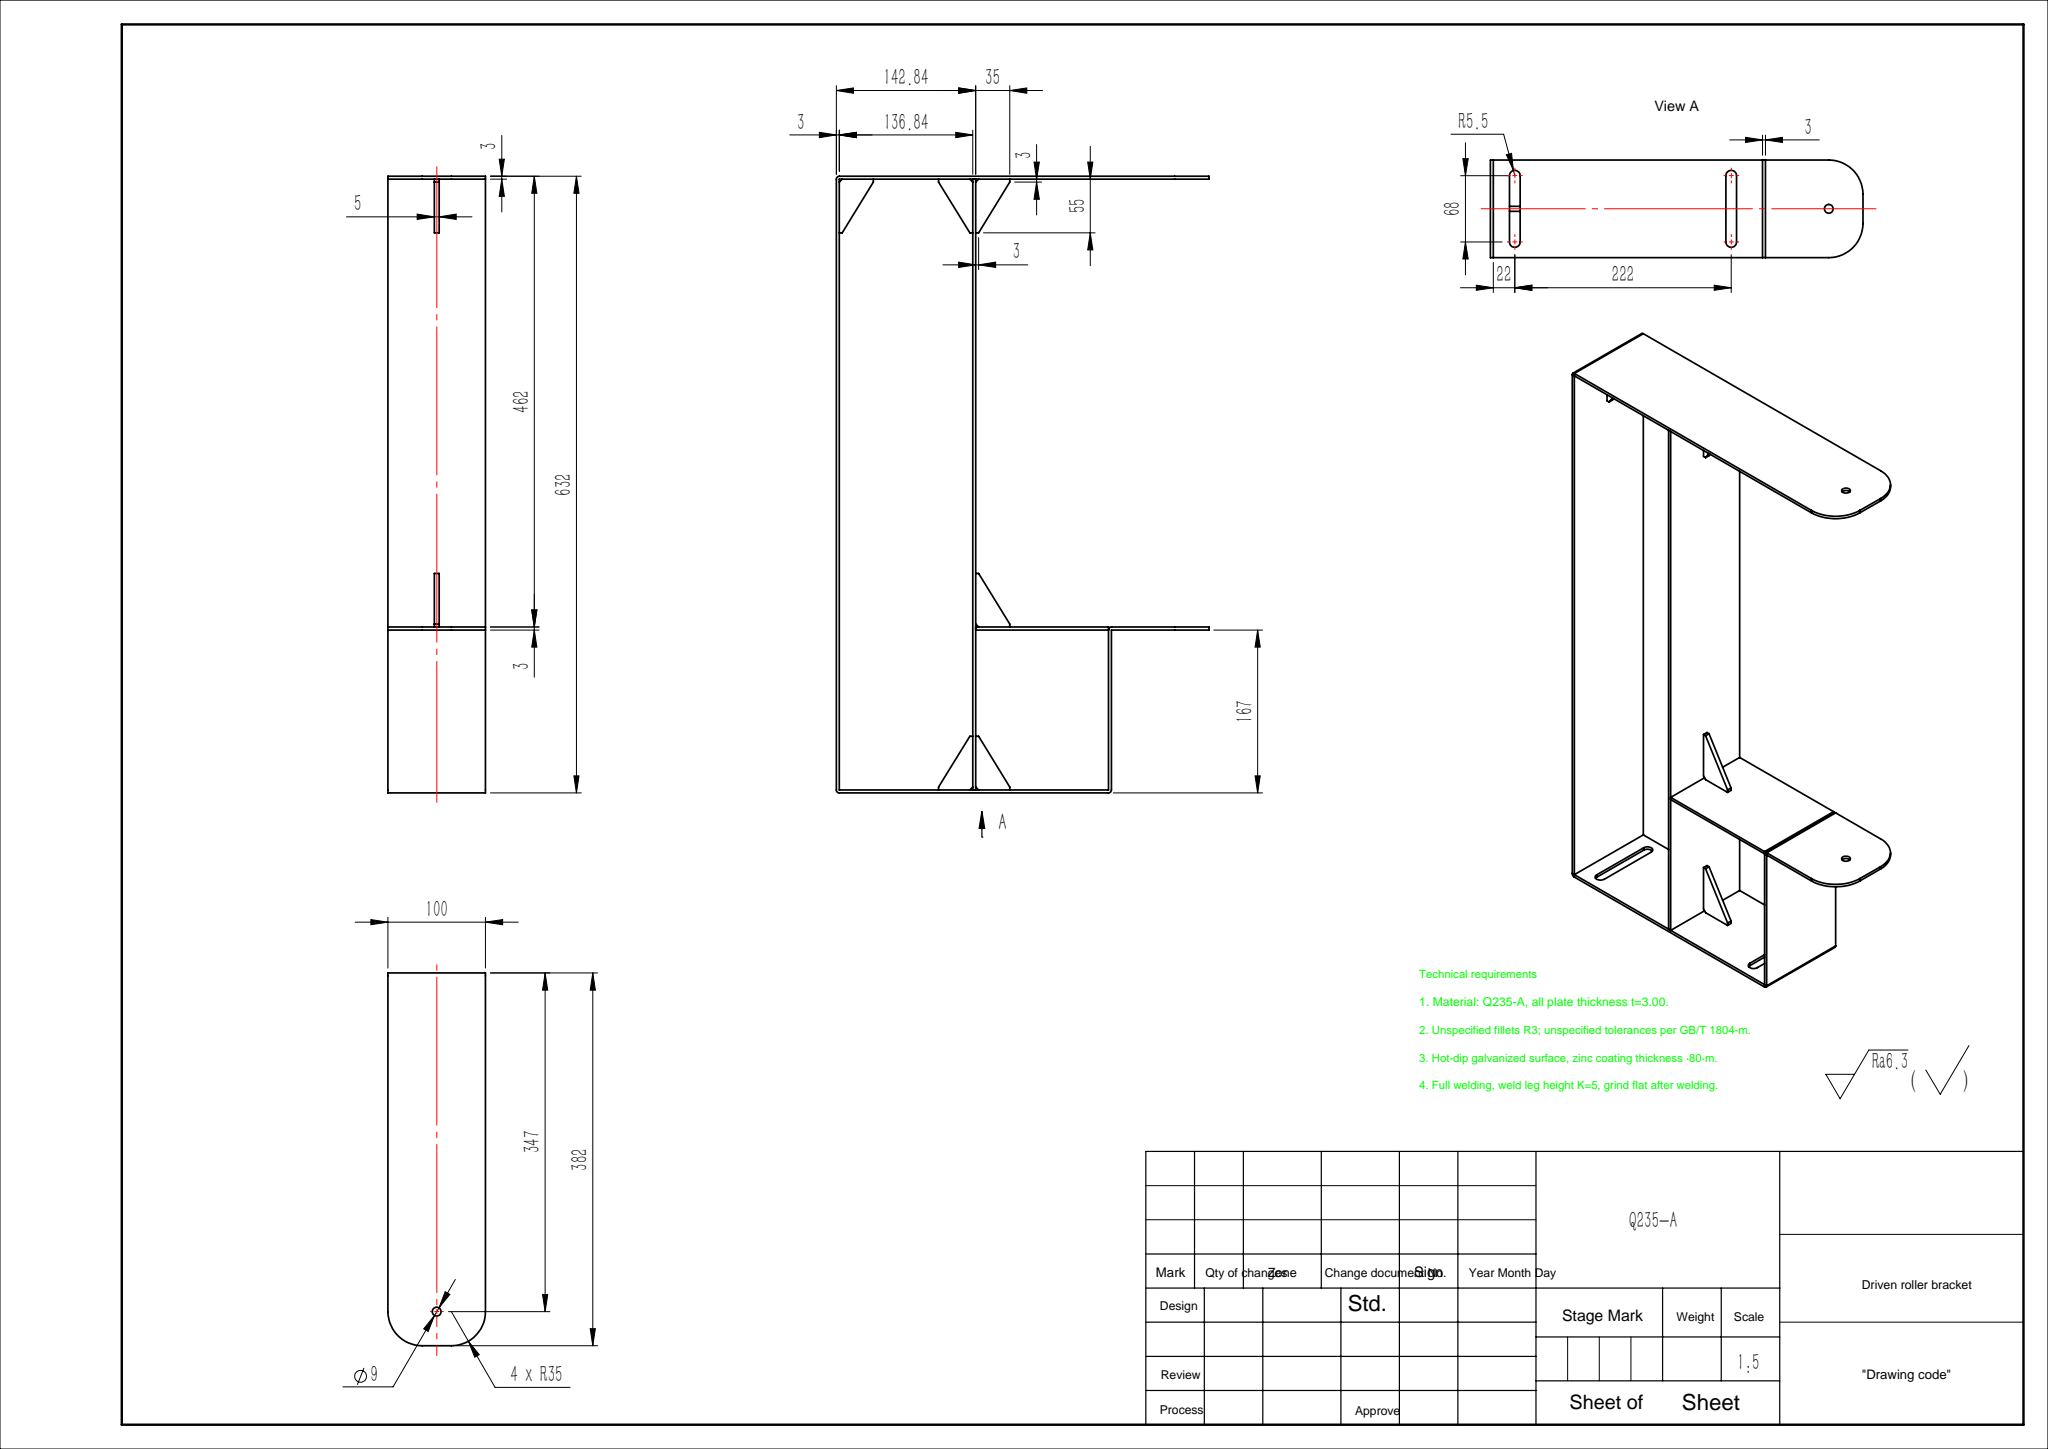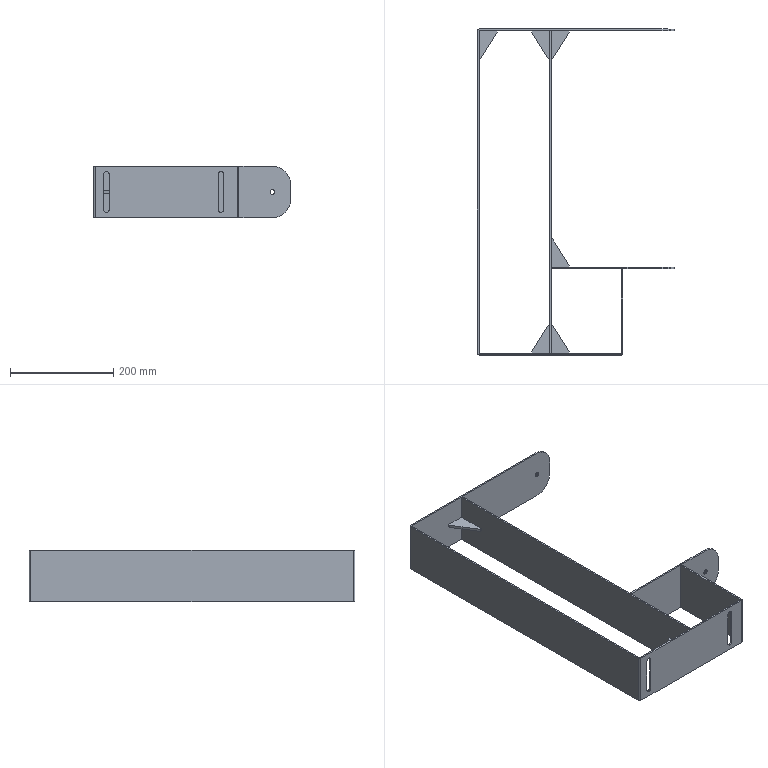Part | SolidWorks | features Gusset 6, FlatPattern 3, SMBaseFlange 3, SheetMetal 3, ICE 2, Fillet 1 | 9 solids | 112 faces | box 382 x 632 x 100 mm | volume 719036 mm3 | plane 94 | cylinder 18 | commonest cylinder face diameters 11 x6 6 x4 9 x4 70 x4